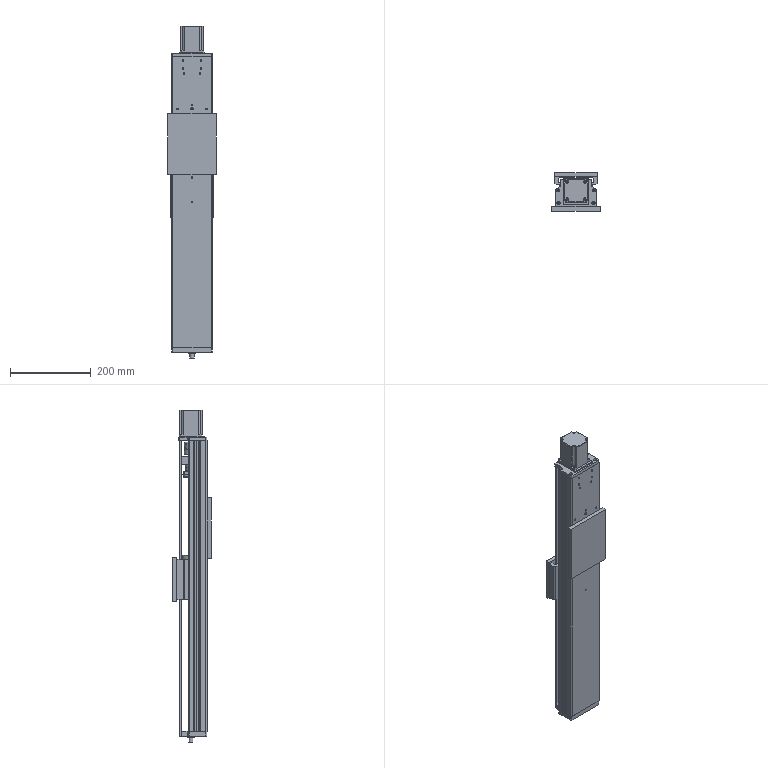Part | NX | 28 solids | 1182 faces | box 120 x 94.5 x 821 mm | volume 2387862 mm3 | plane 451 | cylinder 391 | torus 170 | sphere 78 | cone 76 | spline 16 | commonest cylinder face diameters 8 x36 0.6 x32 4.5 x25 10 x24 3 x22 3.5 x20